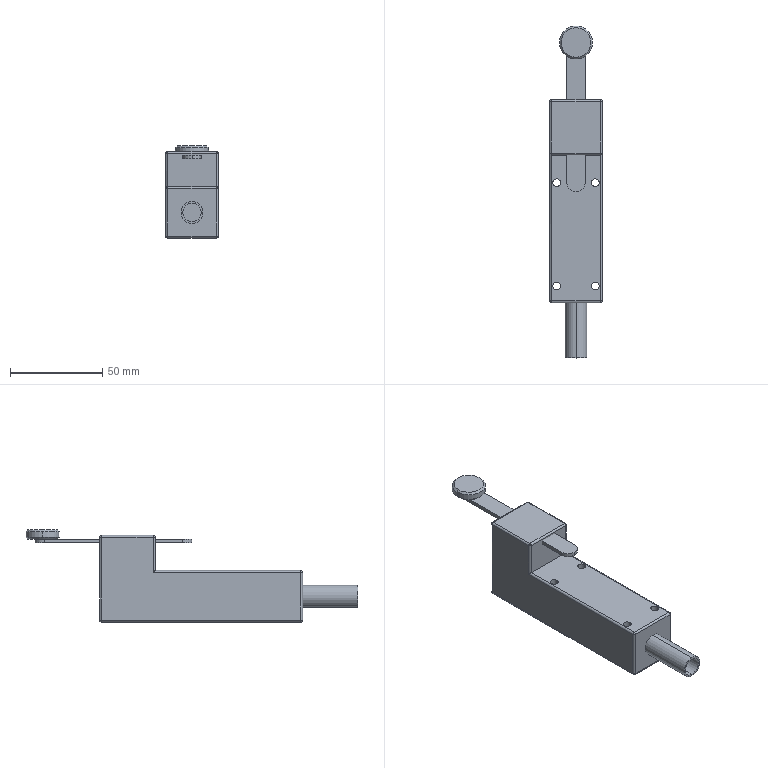Part | STEP file | YBLX-ME-8108 limit switch | 3 solids | 65 faces | box 28.5 x 180 x 50 mm | volume 106221 mm3 | cylinder 35 | plane 16 | sphere 10 | cone 4 | commonest cylinder face diameters 2 x17 4.2 x8 10 x6 12 x2 18 x2